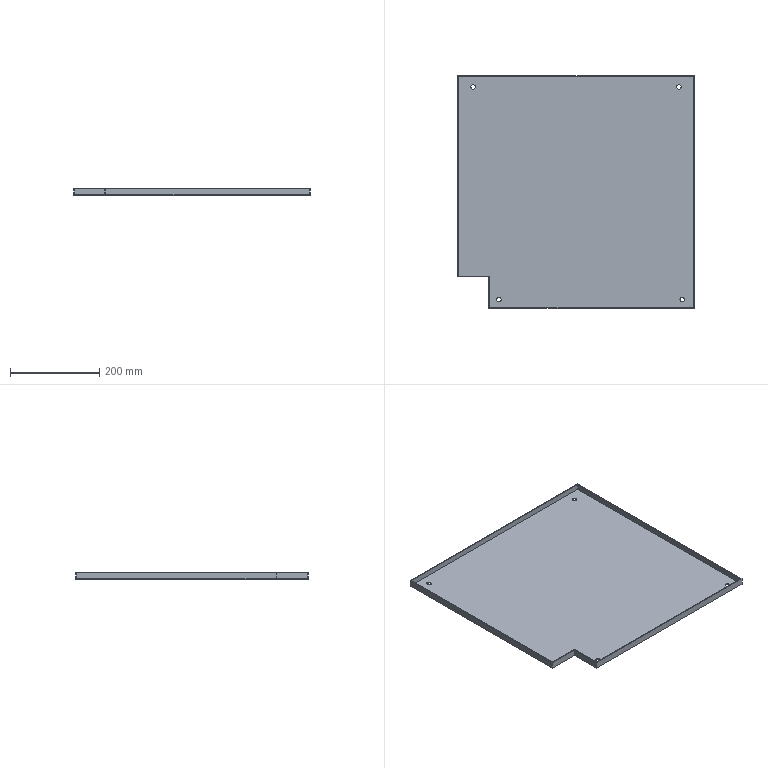Part | STEP file | 11-FGJJ-01411 | 1 solid | 23 faces | box 530 x 520 x 15 mm | volume 595164 mm3 | plane 15 | cylinder 8 | commonest cylinder face diameters 10 x8
STEP:
#1=CARTESIAN_POINT('',(-235.,235.,2.));
#2=VERTEX_POINT('',#1);
#3=CARTESIAN_POINT('',(-225.,235.,2.));
#4=VERTEX_POINT('',#3);
#5=CARTESIAN_POINT('',(-230.,235.,2.));
#6=DIRECTION('',(0.,0.,1.));
#7=DIRECTION('',(1.,0.,0.));
#8=AXIS2_PLACEMENT_3D('',#5,#6,#7);
#9=CIRCLE('',#8,5.);
#10=EDGE_CURVE('',#2,#4,#9,.T.);
#11=ORIENTED_EDGE('',*,*,#10,.T.);
#12=CARTESIAN_POINT('',(-225.,235.,0.));
#13=VERTEX_POINT('',#12);
#14=CARTESIAN_POINT('',(-225.,235.,28.));
#15=DIRECTION('',(0.,0.,-1.));
#16=VECTOR('',#15,1000.);
#17=LINE('',#14,#16);
#18=EDGE_CURVE('',#4,#13,#17,.T.);
#19=ORIENTED_EDGE('',*,*,#18,.T.);
#20=CARTESIAN_POINT('',(-235.,235.,0.));
#21=VERTEX_POINT('',#20);
#22=CARTESIAN_POINT('',(-230.,235.,0.));
#23=DIRECTION('',(0.,0.,-1.));
#24=DIRECTION('',(-1.,0.,0.));
#25=AXIS2_PLACEMENT_3D('',#22,#23,#24);
#26=CIRCLE('',#25,5.);
#27=EDGE_CURVE('',#13,#21,#26,.T.);
#28=ORIENTED_EDGE('',*,*,#27,.T.);
#29=CARTESIAN_POINT('',(-235.,235.,28.));
#30=DIRECTION('',(0.,0.,-1.));
#31=VECTOR('',#30,1000.);
#32=LINE('',#29,#31);
#33=EDGE_CURVE('',#2,#21,#32,.T.);
#34=ORIENTED_EDGE('',*,*,#33,.F.);
#35=EDGE_LOOP('',(#11,#19,#28,#34));
#36=FACE_OUTER_BOUND('',#35,.T.);
#37=CARTESIAN_POINT('',(-230.,235.,28.));
#38=DIRECTION('',(0.,0.,-1.));
#39=DIRECTION('',(-1.,0.,0.));
#40=AXIS2_PLACEMENT_3D('',#37,#38,#39);
#41=CYLINDRICAL_SURFACE('',#40,5.);
#42=ADVANCED_FACE('',(#36),#41,.F.);
#43=CARTESIAN_POINT('',(232.5,-241.,2.));
#44=VERTEX_POINT('',#43);
#45=CARTESIAN_POINT('',(242.5,-241.,2.));
#46=VERTEX_POINT('',#45);
#47=CARTESIAN_POINT('',(237.5,-241.,2.));
#48=DIRECTION('',(0.,0.,1.));
#49=DIRECTION('',(1.,0.,0.));
#50=AXIS2_PLACEMENT_3D('',#47,#48,#49);
#51=CIRCLE('',#50,5.);
#52=EDGE_CURVE('',#44,#46,#51,.T.);
#53=ORIENTED_EDGE('',*,*,#52,.T.);
#54=CARTESIAN_POINT('',(242.5,-241.,0.));
#55=VERTEX_POINT('',#54);
#56=CARTESIAN_POINT('',(242.5,-241.,28.));
#57=DIRECTION('',(0.,0.,-1.));
#58=VECTOR('',#57,1000.);
#59=LINE('',#56,#58);
#60=EDGE_CURVE('',#46,#55,#59,.T.);
#61=ORIENTED_EDGE('',*,*,#60,.T.);
#62=CARTESIAN_POINT('',(232.5,-241.,0.));
#63=VERTEX_POINT('',#62);
#64=CARTESIAN_POINT('',(237.5,-241.,0.));
#65=DIRECTION('',(0.,0.,-1.));
#66=DIRECTION('',(-1.,0.,0.));
#67=AXIS2_PLACEMENT_3D('',#64,#65,#66);
#68=CIRCLE('',#67,5.);
#69=EDGE_CURVE('',#55,#63,#68,.T.);
#70=ORIENTED_EDGE('',*,*,#69,.T.);
#71=CARTESIAN_POINT('',(232.5,-241.,28.));
#72=DIRECTION('',(0.,0.,-1.));
#73=VECTOR('',#72,1000.);
#74=LINE('',#71,#73);
#75=EDGE_CURVE('',#44,#63,#74,.T.);
#76=ORIENTED_EDGE('',*,*,#75,.F.);
#77=EDGE_LOOP('',(#53,#61,#70,#76));
#78=FACE_OUTER_BOUND('',#77,.T.);
#79=CARTESIAN_POINT('',(237.5,-241.,28.));
#80=DIRECTION('',(0.,0.,-1.));
#81=DIRECTION('',(-1.,0.,0.));
#82=AXIS2_PLACEMENT_3D('',#79,#80,#81);
#83=CYLINDRICAL_SURFACE('',#82,5.);
#84=ADVANCED_FACE('',(#78),#83,.F.);
#85=CARTESIAN_POINT('',(-177.5,-241.,2.));
#86=VERTEX_POINT('',#85);
#87=CARTESIAN_POINT('',(-167.5,-241.,2.));
#88=VERTEX_POINT('',#87);
#89=CARTESIAN_POINT('',(-172.5,-241.,2.));
#90=DIRECTION('',(0.,0.,1.));
#91=DIRECTION('',(1.,0.,0.));
#92=AXIS2_PLACEMENT_3D('',#89,#90,#91);
#93=CIRCLE('',#92,5.);
#94=EDGE_CURVE('',#86,#88,#93,.T.);
#95=ORIENTED_EDGE('',*,*,#94,.T.);
#96=CARTESIAN_POINT('',(-167.5,-241.,0.));
#97=VERTEX_POINT('',#96);
#98=CARTESIAN_POINT('',(-167.5,-241.,28.));
#99=DIRECTION('',(0.,0.,-1.));
#100=VECTOR('',#99,1000.);
#101=LINE('',#98,#100);
#102=EDGE_CURVE('',#88,#97,#101,.T.);
#103=ORIENTED_EDGE('',*,*,#102,.T.);
#104=CARTESIAN_POINT('',(-177.5,-241.,0.));
#105=VERTEX_POINT('',#104);
#106=CARTESIAN_POINT('',(-172.5,-241.,0.));
#107=DIRECTION('',(0.,0.,-1.));
#108=DIRECTION('',(-1.,0.,0.));
#109=AXIS2_PLACEMENT_3D('',#106,#107,#108);
#110=CIRCLE('',#109,5.);
#111=EDGE_CURVE('',#97,#105,#110,.T.);
#112=ORIENTED_EDGE('',*,*,#111,.T.);
#113=CARTESIAN_POINT('',(-177.5,-241.,28.));
#114=DIRECTION('',(0.,0.,-1.));
#115=VECTOR('',#114,1000.);
#116=LINE('',#113,#115);
#117=EDGE_CURVE('',#86,#105,#116,.T.);
#118=ORIENTED_EDGE('',*,*,#117,.F.);
#119=EDGE_LOOP('',(#95,#103,#112,#118));
#120=FACE_OUTER_BOUND('',#119,.T.);
#121=CARTESIAN_POINT('',(-172.5,-241.,28.));
#122=DIRECTION('',(0.,0.,-1.));
#123=DIRECTION('',(-1.,0.,0.));
#124=AXIS2_PLACEMENT_3D('',#121,#122,#123);
#125=CYLINDRICAL_SURFACE('',#124,5.);
#126=ADVANCED_FACE('',(#120),#125,.F.);
#127=CARTESIAN_POINT('',(225.,235.,2.));
#128=VERTEX_POINT('',#127);
#129=CARTESIAN_POINT('',(235.,235.,2.));
#130=VERTEX_POINT('',#129);
#131=CARTESIAN_POINT('',(230.,235.,2.));
#132=DIRECTION('',(0.,0.,1.));
#133=DIRECTION('',(1.,0.,0.));
#134=AXIS2_PLACEMENT_3D('',#131,#132,#133);
#135=CIRCLE('',#134,5.);
#136=EDGE_CURVE('',#128,#130,#135,.T.);
#137=ORIENTED_EDGE('',*,*,#136,.T.);
#138=CARTESIAN_POINT('',(235.,235.,0.));
#139=VERTEX_POINT('',#138);
#140=CARTESIAN_POINT('',(235.,235.,28.));
#141=DIRECTION('',(0.,0.,-1.));
#142=VECTOR('',#141,1000.);
#143=LINE('',#140,#142);
#144=EDGE_CURVE('',#130,#139,#143,.T.);
#145=ORIENTED_EDGE('',*,*,#144,.T.);
#146=CARTESIAN_POINT('',(225.,235.,0.));
#147=VERTEX_POINT('',#146);
#148=CARTESIAN_POINT('',(230.,235.,0.));
#149=DIRECTION('',(0.,0.,-1.));
#150=DIRECTION('',(-1.,0.,0.));
#151=AXIS2_PLACEMENT_3D('',#148,#149,#150);
#152=CIRCLE('',#151,5.);
#153=EDGE_CURVE('',#139,#147,#152,.T.);
#154=ORIENTED_EDGE('',*,*,#153,.T.);
#155=CARTESIAN_POINT('',(225.,235.,28.));
#156=DIRECTION('',(0.,0.,-1.));
#157=VECTOR('',#156,1000.);
#158=LINE('',#155,#157);
#159=EDGE_CURVE('',#128,#147,#158,.T.);
#160=ORIENTED_EDGE('',*,*,#159,.F.);
#161=EDGE_LOOP('',(#137,#145,#154,#160));
#162=FACE_OUTER_BOUND('',#161,.T.);
#163=CARTESIAN_POINT('',(230.,235.,28.));
#164=DIRECTION('',(0.,0.,-1.));
#165=DIRECTION('',(-1.,0.,0.));
#166=AXIS2_PLACEMENT_3D('',#163,#164,#165);
#167=CYLINDRICAL_SURFACE('',#166,5.);
#168=ADVANCED_FACE('',(#162),#167,.F.);
#169=CARTESIAN_POINT('',(-263.,258.,15.));
#170=VERTEX_POINT('',#169);
#171=CARTESIAN_POINT('',(-263.,-188.,15.));
#172=VERTEX_POINT('',#171);
#173=CARTESIAN_POINT('',(-263.,260.,15.));
#174=DIRECTION('',(0.,-1.,0.));
#175=VECTOR('',#174,1000.);
#176=LINE('',#173,#175);
#177=EDGE_CURVE('',#170,#172,#176,.T.);
#178=ORIENTED_EDGE('',*,*,#177,.T.);
#179=CARTESIAN_POINT('',(-263.,-188.,2.));
#180=VERTEX_POINT('',#179);
#181=CARTESIAN_POINT('',(-263.,-188.,113.995));
#182=DIRECTION('',(0.,0.,-1.));
#183=VECTOR('',#182,1000.);
#184=LINE('',#181,#183);
#185=EDGE_CURVE('',#172,#180,#184,.T.);
#186=ORIENTED_EDGE('',*,*,#185,.T.);
#187=CARTESIAN_POINT('',(-263.,258.,2.));
#188=VERTEX_POINT('',#187);
#189=CARTESIAN_POINT('',(-263.,260.,2.));
#190=DIRECTION('',(0.,-1.,0.));
#191=VECTOR('',#190,1000.);
#192=LINE('',#189,#191);
#193=EDGE_CURVE('',#188,#180,#192,.T.);
#194=ORIENTED_EDGE('',*,*,#193,.F.);
#195=CARTESIAN_POINT('',(-263.,258.,15.));
#196=DIRECTION('',(0.,0.,-1.));
#197=VECTOR('',#196,1000.);
#198=LINE('',#195,#197);
#199=EDGE_CURVE('',#170,#188,#198,.T.);
#200=ORIENTED_EDGE('',*,*,#199,.F.);
#201=EDGE_LOOP('',(#178,#186,#194,#200));
#202=FACE_OUTER_BOUND('',#201,.T.);
#203=CARTESIAN_POINT('',(-263.,260.,15.));
#204=DIRECTION('',(1.,0.,0.));
#205=DIRECTION('',(0.,1.,0.));
#206=AXIS2_PLACEMENT_3D('',#203,#204,#205);
#207=PLANE('',#206);
#208=ADVANCED_FACE('',(#202),#207,.T.);
#209=CARTESIAN_POINT('',(-193.,-258.,2.));
#210=VERTEX_POINT('',#209);
#211=CARTESIAN_POINT('',(263.,-258.,2.));
#212=VERTEX_POINT('',#211);
#213=CARTESIAN_POINT('',(-265.,-258.,2.));
#214=DIRECTION('',(1.,0.,0.));
#215=VECTOR('',#214,1000.);
#216=LINE('',#213,#215);
#217=EDGE_CURVE('',#210,#212,#216,.T.);
#218=ORIENTED_EDGE('',*,*,#217,.F.);
#219=CARTESIAN_POINT('',(-193.,-258.,15.));
#220=VERTEX_POINT('',#219);
#221=CARTESIAN_POINT('',(-193.,-258.,113.995));
#222=DIRECTION('',(0.,0.,-1.));
#223=VECTOR('',#222,1000.);
#224=LINE('',#221,#223);
#225=EDGE_CURVE('',#220,#210,#224,.T.);
#226=ORIENTED_EDGE('',*,*,#225,.F.);
#227=CARTESIAN_POINT('',(263.,-258.,15.));
#228=VERTEX_POINT('',#227);
#229=CARTESIAN_POINT('',(-265.,-258.,15.));
#230=DIRECTION('',(1.,0.,0.));
#231=VECTOR('',#230,1000.);
#232=LINE('',#229,#231);
#233=EDGE_CURVE('',#220,#228,#232,.T.);
#234=ORIENTED_EDGE('',*,*,#233,.T.);
#235=CARTESIAN_POINT('',(263.,-258.,15.));
#236=DIRECTION('',(0.,0.,-1.));
#237=VECTOR('',#236,1000.);
#238=LINE('',#235,#237);
#239=EDGE_CURVE('',#228,#212,#238,.T.);
#240=ORIENTED_EDGE('',*,*,#239,.T.);
#241=EDGE_LOOP('',(#218,#226,#234,#240));
#242=FACE_OUTER_BOUND('',#241,.T.);
#243=CARTESIAN_POINT('',(-265.,-258.,15.));
#244=DIRECTION('',(0.,1.,0.));
#245=DIRECTION('',(0.,0.,1.));
#246=AXIS2_PLACEMENT_3D('',#243,#244,#245);
#247=PLANE('',#246);
#248=ADVANCED_FACE('',(#242),#247,.T.);
#249=ORIENTED_EDGE('',*,*,#10,.F.);
#250=CARTESIAN_POINT('',(-230.,235.,2.));
#251=DIRECTION('',(0.,0.,1.));
#252=DIRECTION('',(1.,0.,0.));
#253=AXIS2_PLACEMENT_3D('',#250,#251,#252);
#254=CIRCLE('',#253,5.);
#255=EDGE_CURVE('',#4,#2,#254,.T.);
#256=ORIENTED_EDGE('',*,*,#255,.F.);
#257=EDGE_LOOP('',(#249,#256));
#258=FACE_BOUND('',#257,.T.);
#259=ORIENTED_EDGE('',*,*,#52,.F.);
#260=CARTESIAN_POINT('',(237.5,-241.,2.));
#261=DIRECTION('',(0.,0.,1.));
#262=DIRECTION('',(1.,0.,0.));
#263=AXIS2_PLACEMENT_3D('',#260,#261,#262);
#264=CIRCLE('',#263,5.);
#265=EDGE_CURVE('',#46,#44,#264,.T.);
#266=ORIENTED_EDGE('',*,*,#265,.F.);
#267=EDGE_LOOP('',(#259,#266));
#268=FACE_BOUND('',#267,.T.);
#269=ORIENTED_EDGE('',*,*,#94,.F.);
#270=CARTESIAN_POINT('',(-172.5,-241.,2.));
#271=DIRECTION('',(0.,0.,1.));
#272=DIRECTION('',(1.,0.,0.));
#273=AXIS2_PLACEMENT_3D('',#270,#271,#272);
#274=CIRCLE('',#273,5.);
#275=EDGE_CURVE('',#88,#86,#274,.T.);
#276=ORIENTED_EDGE('',*,*,#275,.F.);
#277=EDGE_LOOP('',(#269,#276));
#278=FACE_BOUND('',#277,.T.);
#279=ORIENTED_EDGE('',*,*,#136,.F.);
#280=CARTESIAN_POINT('',(230.,235.,2.));
#281=DIRECTION('',(0.,0.,1.));
#282=DIRECTION('',(1.,0.,0.));
#283=AXIS2_PLACEMENT_3D('',#280,#281,#282);
#284=CIRCLE('',#283,5.);
#285=EDGE_CURVE('',#130,#128,#284,.T.);
#286=ORIENTED_EDGE('',*,*,#285,.F.);
#287=EDGE_LOOP('',(#279,#286));
#288=FACE_BOUND('',#287,.T.);
#289=CARTESIAN_POINT('',(-193.,-188.,2.));
#290=VERTEX_POINT('',#289);
#291=CARTESIAN_POINT('',(-263.,-188.,2.));
#292=DIRECTION('',(-1.,0.,0.));
#293=VECTOR('',#292,1000.);
#294=LINE('',#291,#293);
#295=EDGE_CURVE('',#290,#180,#294,.T.);
#296=ORIENTED_EDGE('',*,*,#295,.F.);
#297=CARTESIAN_POINT('',(-193.,-258.,2.));
#298=DIRECTION('',(0.,1.,0.));
#299=VECTOR('',#298,1000.);
#300=LINE('',#297,#299);
#301=EDGE_CURVE('',#210,#290,#300,.T.);
#302=ORIENTED_EDGE('',*,*,#301,.F.);
#303=ORIENTED_EDGE('',*,*,#217,.T.);
#304=CARTESIAN_POINT('',(263.,258.,2.));
#305=VERTEX_POINT('',#304);
#306=CARTESIAN_POINT('',(263.,260.,2.));
#307=DIRECTION('',(0.,1.,0.));
#308=VECTOR('',#307,1000.);
#309=LINE('',#306,#308);
#310=EDGE_CURVE('',#212,#305,#309,.T.);
#311=ORIENTED_EDGE('',*,*,#310,.T.);
#312=CARTESIAN_POINT('',(-265.,258.,2.));
#313=DIRECTION('',(-1.,0.,0.));
#314=VECTOR('',#313,1000.);
#315=LINE('',#312,#314);
#316=EDGE_CURVE('',#305,#188,#315,.T.);
#317=ORIENTED_EDGE('',*,*,#316,.T.);
#318=ORIENTED_EDGE('',*,*,#193,.T.);
#319=EDGE_LOOP('',(#296,#302,#303,#311,#317,#318));
#320=FACE_OUTER_BOUND('',#319,.T.);
#321=CARTESIAN_POINT('',(0.,0.,2.));
#322=DIRECTION('',(0.,0.,1.));
#323=DIRECTION('',(1.,0.,0.));
#324=AXIS2_PLACEMENT_3D('',#321,#322,#323);
#325=PLANE('',#324);
#326=ADVANCED_FACE('',(#258,#268,#278,#288,#320),#325,.T.);
#327=CARTESIAN_POINT('',(265.,-260.,0.));
#328=VERTEX_POINT('',#327);
#329=CARTESIAN_POINT('',(265.,260.,0.));
#330=VERTEX_POINT('',#329);
#331=CARTESIAN_POINT('',(265.,260.,0.));
#332=DIRECTION('',(0.,1.,0.));
#333=VECTOR('',#332,1000.);
#334=LINE('',#331,#333);
#335=EDGE_CURVE('',#328,#330,#334,.T.);
#336=ORIENTED_EDGE('',*,*,#335,.T.);
#337=CARTESIAN_POINT('',(265.,260.,15.));
#338=VERTEX_POINT('',#337);
#339=CARTESIAN_POINT('',(265.,260.,15.));
#340=DIRECTION('',(0.,0.,-1.));
#341=VECTOR('',#340,1000.);
#342=LINE('',#339,#341);
#343=EDGE_CURVE('',#338,#330,#342,.T.);
#344=ORIENTED_EDGE('',*,*,#343,.F.);
#345=CARTESIAN_POINT('',(265.,-260.,15.));
#346=VERTEX_POINT('',#345);
#347=CARTESIAN_POINT('',(265.,260.,15.));
#348=DIRECTION('',(0.,1.,0.));
#349=VECTOR('',#348,1000.);
#350=LINE('',#347,#349);
#351=EDGE_CURVE('',#346,#338,#350,.T.);
#352=ORIENTED_EDGE('',*,*,#351,.F.);
#353=CARTESIAN_POINT('',(265.,-260.,15.));
#354=DIRECTION('',(0.,0.,-1.));
#355=VECTOR('',#354,1000.);
#356=LINE('',#353,#355);
#357=EDGE_CURVE('',#346,#328,#356,.T.);
#358=ORIENTED_EDGE('',*,*,#357,.T.);
#359=EDGE_LOOP('',(#336,#344,#352,#358));
#360=FACE_OUTER_BOUND('',#359,.T.);
#361=CARTESIAN_POINT('',(265.,260.,15.));
#362=DIRECTION('',(-1.,0.,0.));
#363=DIRECTION('',(0.,-1.,0.));
#364=AXIS2_PLACEMENT_3D('',#361,#362,#363);
#365=PLANE('',#364);
#366=ADVANCED_FACE('',(#360),#365,.F.);
#367=CARTESIAN_POINT('',(-265.,260.,0.));
#368=VERTEX_POINT('',#367);
#369=CARTESIAN_POINT('',(-265.,260.,0.));
#370=DIRECTION('',(-1.,0.,0.));
#371=VECTOR('',#370,1000.);
#372=LINE('',#369,#371);
#373=EDGE_CURVE('',#330,#368,#372,.T.);
#374=ORIENTED_EDGE('',*,*,#373,.T.);
#375=CARTESIAN_POINT('',(-265.,260.,15.));
#376=VERTEX_POINT('',#375);
#377=CARTESIAN_POINT('',(-265.,260.,15.));
#378=DIRECTION('',(0.,0.,-1.));
#379=VECTOR('',#378,1000.);
#380=LINE('',#377,#379);
#381=EDGE_CURVE('',#376,#368,#380,.T.);
#382=ORIENTED_EDGE('',*,*,#381,.F.);
#383=CARTESIAN_POINT('',(-265.,260.,15.));
#384=DIRECTION('',(-1.,0.,0.));
#385=VECTOR('',#384,1000.);
#386=LINE('',#383,#385);
#387=EDGE_CURVE('',#338,#376,#386,.T.);
#388=ORIENTED_EDGE('',*,*,#387,.F.);
#389=ORIENTED_EDGE('',*,*,#343,.T.);
#390=EDGE_LOOP('',(#374,#382,#388,#389));
#391=FACE_OUTER_BOUND('',#390,.T.);
#392=CARTESIAN_POINT('',(-265.,260.,15.));
#393=DIRECTION('',(0.,-1.,0.));
#394=DIRECTION('',(0.,0.,-1.));
#395=AXIS2_PLACEMENT_3D('',#392,#393,#394);
#396=PLANE('',#395);
#397=ADVANCED_FACE('',(#391),#396,.F.);
#398=CARTESIAN_POINT('',(-265.,-190.,0.));
#399=VERTEX_POINT('',#398);
#400=CARTESIAN_POINT('',(-265.,260.,0.));
#401=DIRECTION('',(0.,-1.,0.));
#402=VECTOR('',#401,1000.);
#403=LINE('',#400,#402);
#404=EDGE_CURVE('',#368,#399,#403,.T.);
#405=ORIENTED_EDGE('',*,*,#404,.T.);
#406=CARTESIAN_POINT('',(-265.,-190.,15.));
#407=VERTEX_POINT('',#406);
#408=CARTESIAN_POINT('',(-265.,-190.,28.));
#409=DIRECTION('',(0.,0.,-1.));
#410=VECTOR('',#409,1000.);
#411=LINE('',#408,#410);
#412=EDGE_CURVE('',#407,#399,#411,.T.);
#413=ORIENTED_EDGE('',*,*,#412,.F.);
#414=CARTESIAN_POINT('',(-265.,260.,15.));
#415=DIRECTION('',(0.,-1.,0.));
#416=VECTOR('',#415,1000.);
#417=LINE('',#414,#416);
#418=EDGE_CURVE('',#376,#407,#417,.T.);
#419=ORIENTED_EDGE('',*,*,#418,.F.);
#420=ORIENTED_EDGE('',*,*,#381,.T.);
#421=EDGE_LOOP('',(#405,#413,#419,#420));
#422=FACE_OUTER_BOUND('',#421,.T.);
#423=CARTESIAN_POINT('',(-265.,260.,15.));
#424=DIRECTION('',(1.,0.,0.));
#425=DIRECTION('',(0.,1.,0.));
#426=AXIS2_PLACEMENT_3D('',#423,#424,#425);
#427=PLANE('',#426);
#428=ADVANCED_FACE('',(#422),#427,.F.);
#429=CARTESIAN_POINT('',(-195.,-260.,15.));
#430=VERTEX_POINT('',#429);
#431=CARTESIAN_POINT('',(-265.,-260.,15.));
#432=DIRECTION('',(1.,0.,0.));
#433=VECTOR('',#432,1000.);
#434=LINE('',#431,#433);
#435=EDGE_CURVE('',#430,#346,#434,.T.);
#436=ORIENTED_EDGE('',*,*,#435,.F.);
#437=CARTESIAN_POINT('',(-195.,-260.,0.));
#438=VERTEX_POINT('',#437);
#439=CARTESIAN_POINT('',(-195.,-260.,28.));
#440=DIRECTION('',(0.,0.,-1.));
#441=VECTOR('',#440,1000.);
#442=LINE('',#439,#441);
#443=EDGE_CURVE('',#430,#438,#442,.T.);
#444=ORIENTED_EDGE('',*,*,#443,.T.);
#445=CARTESIAN_POINT('',(-265.,-260.,0.));
#446=DIRECTION('',(1.,0.,0.));
#447=VECTOR('',#446,1000.);
#448=LINE('',#445,#447);
#449=EDGE_CURVE('',#438,#328,#448,.T.);
#450=ORIENTED_EDGE('',*,*,#449,.T.);
#451=ORIENTED_EDGE('',*,*,#357,.F.);
#452=EDGE_LOOP('',(#436,#444,#450,#451));
#453=FACE_OUTER_BOUND('',#452,.T.);
#454=CARTESIAN_POINT('',(-265.,-260.,15.));
#455=DIRECTION('',(0.,1.,0.));
#456=DIRECTION('',(0.,0.,1.));
#457=AXIS2_PLACEMENT_3D('',#454,#455,#456);
#458=PLANE('',#457);
#459=ADVANCED_FACE('',(#453),#458,.F.);
#460=CARTESIAN_POINT('',(-195.,-190.,15.));
#461=VERTEX_POINT('',#460);
#462=CARTESIAN_POINT('',(0.,-190.,15.));
#463=DIRECTION('',(-1.,0.,0.));
#464=VECTOR('',#463,1000.);
#465=LINE('',#462,#464);
#466=EDGE_CURVE('',#461,#407,#465,.T.);
#467=ORIENTED_EDGE('',*,*,#466,.F.);
#468=CARTESIAN_POINT('',(-195.,0.,15.));
#469=DIRECTION('',(0.,1.,0.));
#470=VECTOR('',#469,1000.);
#471=LINE('',#468,#470);
#472=EDGE_CURVE('',#430,#461,#471,.T.);
#473=ORIENTED_EDGE('',*,*,#472,.F.);
#474=ORIENTED_EDGE('',*,*,#435,.T.);
#475=ORIENTED_EDGE('',*,*,#351,.T.);
#476=ORIENTED_EDGE('',*,*,#387,.T.);
#477=ORIENTED_EDGE('',*,*,#418,.T.);
#478=EDGE_LOOP('',(#467,#473,#474,#475,#476,#477));
#479=FACE_OUTER_BOUND('',#478,.T.);
#480=CARTESIAN_POINT('',(-193.,-188.,15.));
#481=VERTEX_POINT('',#480);
#482=CARTESIAN_POINT('',(-263.,-188.,15.));
#483=DIRECTION('',(-1.,0.,0.));
#484=VECTOR('',#483,1000.);
#485=LINE('',#482,#484);
#486=EDGE_CURVE('',#481,#172,#485,.T.);
#487=ORIENTED_EDGE('',*,*,#486,.T.);
#488=ORIENTED_EDGE('',*,*,#177,.F.);
#489=CARTESIAN_POINT('',(263.,258.,15.));
#490=VERTEX_POINT('',#489);
#491=CARTESIAN_POINT('',(-265.,258.,15.));
#492=DIRECTION('',(-1.,0.,0.));
#493=VECTOR('',#492,1000.);
#494=LINE('',#491,#493);
#495=EDGE_CURVE('',#490,#170,#494,.T.);
#496=ORIENTED_EDGE('',*,*,#495,.F.);
#497=CARTESIAN_POINT('',(263.,260.,15.));
#498=DIRECTION('',(0.,1.,0.));
#499=VECTOR('',#498,1000.);
#500=LINE('',#497,#499);
#501=EDGE_CURVE('',#228,#490,#500,.T.);
#502=ORIENTED_EDGE('',*,*,#501,.F.);
#503=ORIENTED_EDGE('',*,*,#233,.F.);
#504=CARTESIAN_POINT('',(-193.,-258.,15.));
#505=DIRECTION('',(0.,1.,0.));
#506=VECTOR('',#505,1000.);
#507=LINE('',#504,#506);
#508=EDGE_CURVE('',#220,#481,#507,.T.);
#509=ORIENTED_EDGE('',*,*,#508,.T.);
#510=EDGE_LOOP('',(#487,#488,#496,#502,#503,#509));
#511=FACE_BOUND('',#510,.T.);
#512=CARTESIAN_POINT('',(0.,0.,15.));
#513=DIRECTION('',(0.,0.,1.));
#514=DIRECTION('',(1.,0.,0.));
#515=AXIS2_PLACEMENT_3D('',#512,#513,#514);
#516=PLANE('',#515);
#517=ADVANCED_FACE('',(#479,#511),#516,.T.);
#518=CARTESIAN_POINT('',(-230.,235.,0.));
#519=DIRECTION('',(0.,0.,-1.));
#520=DIRECTION('',(-1.,0.,0.));
#521=AXIS2_PLACEMENT_3D('',#518,#519,#520);
#522=CIRCLE('',#521,5.);
#523=EDGE_CURVE('',#21,#13,#522,.T.);
#524=ORIENTED_EDGE('',*,*,#523,.F.);
#525=ORIENTED_EDGE('',*,*,#27,.F.);
#526=EDGE_LOOP('',(#524,#525));
#527=FACE_BOUND('',#526,.T.);
#528=CARTESIAN_POINT('',(237.5,-241.,0.));
#529=DIRECTION('',(0.,0.,-1.));
#530=DIRECTION('',(-1.,0.,0.));
#531=AXIS2_PLACEMENT_3D('',#528,#529,#530);
#532=CIRCLE('',#531,5.);
#533=EDGE_CURVE('',#63,#55,#532,.T.);
#534=ORIENTED_EDGE('',*,*,#533,.F.);
#535=ORIENTED_EDGE('',*,*,#69,.F.);
#536=EDGE_LOOP('',(#534,#535));
#537=FACE_BOUND('',#536,.T.);
#538=CARTESIAN_POINT('',(-172.5,-241.,0.));
#539=DIRECTION('',(0.,0.,-1.));
#540=DIRECTION('',(-1.,0.,0.));
#541=AXIS2_PLACEMENT_3D('',#538,#539,#540);
#542=CIRCLE('',#541,5.);
#543=EDGE_CURVE('',#105,#97,#542,.T.);
#544=ORIENTED_EDGE('',*,*,#543,.F.);
#545=ORIENTED_EDGE('',*,*,#111,.F.);
#546=EDGE_LOOP('',(#544,#545));
#547=FACE_BOUND('',#546,.T.);
#548=CARTESIAN_POINT('',(230.,235.,0.));
#549=DIRECTION('',(0.,0.,-1.));
#550=DIRECTION('',(-1.,0.,0.));
#551=AXIS2_PLACEMENT_3D('',#548,#549,#550);
#552=CIRCLE('',#551,5.);
#553=EDGE_CURVE('',#147,#139,#552,.T.);
#554=ORIENTED_EDGE('',*,*,#553,.F.);
#555=ORIENTED_EDGE('',*,*,#153,.F.);
#556=EDGE_LOOP('',(#554,#555));
#557=FACE_BOUND('',#556,.T.);
#558=ORIENTED_EDGE('',*,*,#449,.F.);
#559=CARTESIAN_POINT('',(-195.,-190.,0.));
#560=VERTEX_POINT('',#559);
#561=CARTESIAN_POINT('',(-195.,-260.,0.));
#562=DIRECTION('',(0.,-1.,0.));
#563=VECTOR('',#562,1000.);
#564=LINE('',#561,#563);
#565=EDGE_CURVE('',#560,#438,#564,.T.);
#566=ORIENTED_EDGE('',*,*,#565,.F.);
#567=CARTESIAN_POINT('',(-265.,-190.,0.));
#568=DIRECTION('',(1.,0.,0.));
#569=VECTOR('',#568,1000.);
#570=LINE('',#567,#569);
#571=EDGE_CURVE('',#399,#560,#570,.T.);
#572=ORIENTED_EDGE('',*,*,#571,.F.);
#573=ORIENTED_EDGE('',*,*,#404,.F.);
#574=ORIENTED_EDGE('',*,*,#373,.F.);
#575=ORIENTED_EDGE('',*,*,#335,.F.);
#576=EDGE_LOOP('',(#558,#566,#572,#573,#574,#575));
#577=FACE_OUTER_BOUND('',#576,.T.);
#578=CARTESIAN_POINT('',(0.,0.,0.));
#579=DIRECTION('',(0.,0.,1.));
#580=DIRECTION('',(1.,0.,0.));
#581=AXIS2_PLACEMENT_3D('',#578,#579,#580);
#582=PLANE('',#581);
#583=ADVANCED_FACE('',(#527,#537,#547,#557,#577),#582,.F.);
#584=ORIENTED_EDGE('',*,*,#310,.F.);
#585=ORIENTED_EDGE('',*,*,#239,.F.);
#586=ORIENTED_EDGE('',*,*,#501,.T.);
#587=CARTESIAN_POINT('',(263.,258.,15.));
#588=DIRECTION('',(0.,0.,-1.));
#589=VECTOR('',#588,1000.);
#590=LINE('',#587,#589);
#591=EDGE_CURVE('',#490,#305,#590,.T.);
#592=ORIENTED_EDGE('',*,*,#591,.T.);
#593=EDGE_LOOP('',(#584,#585,#586,#592));
#594=FACE_OUTER_BOUND('',#593,.T.);
#595=CARTESIAN_POINT('',(263.,260.,15.));
#596=DIRECTION('',(-1.,0.,0.));
#597=DIRECTION('',(0.,-1.,0.));
#598=AXIS2_PLACEMENT_3D('',#595,#596,#597);
#599=PLANE('',#598);
#600=ADVANCED_FACE('',(#594),#599,.T.);
#601=ORIENTED_EDGE('',*,*,#316,.F.);
#602=ORIENTED_EDGE('',*,*,#591,.F.);
#603=ORIENTED_EDGE('',*,*,#495,.T.);
#604=ORIENTED_EDGE('',*,*,#199,.T.);
#605=EDGE_LOOP('',(#601,#602,#603,#604));
#606=FACE_OUTER_BOUND('',#605,.T.);
#607=CARTESIAN_POINT('',(-265.,258.,15.));
#608=DIRECTION('',(0.,-1.,0.));
#609=DIRECTION('',(0.,0.,-1.));
#610=AXIS2_PLACEMENT_3D('',#607,#608,#609);
#611=PLANE('',#610);
#612=ADVANCED_FACE('',(#606),#611,.T.);
#613=ORIENTED_EDGE('',*,*,#144,.F.);
#614=ORIENTED_EDGE('',*,*,#285,.T.);
#615=ORIENTED_EDGE('',*,*,#159,.T.);
#616=ORIENTED_EDGE('',*,*,#553,.T.);
#617=EDGE_LOOP('',(#613,#614,#615,#616));
#618=FACE_OUTER_BOUND('',#617,.T.);
#619=CARTESIAN_POINT('',(230.,235.,28.));
#620=DIRECTION('',(0.,0.,-1.));
#621=DIRECTION('',(-1.,0.,0.));
#622=AXIS2_PLACEMENT_3D('',#619,#620,#621);
#623=CYLINDRICAL_SURFACE('',#622,5.);
#624=ADVANCED_FACE('',(#618),#623,.F.);
#625=ORIENTED_EDGE('',*,*,#102,.F.);
#626=ORIENTED_EDGE('',*,*,#275,.T.);
#627=ORIENTED_EDGE('',*,*,#117,.T.);
#628=ORIENTED_EDGE('',*,*,#543,.T.);
#629=EDGE_LOOP('',(#625,#626,#627,#628));
#630=FACE_OUTER_BOUND('',#629,.T.);
#631=CARTESIAN_POINT('',(-172.5,-241.,28.));
#632=DIRECTION('',(0.,0.,-1.));
#633=DIRECTION('',(-1.,0.,0.));
#634=AXIS2_PLACEMENT_3D('',#631,#632,#633);
#635=CYLINDRICAL_SURFACE('',#634,5.);
#636=ADVANCED_FACE('',(#630),#635,.F.);
#637=ORIENTED_EDGE('',*,*,#60,.F.);
#638=ORIENTED_EDGE('',*,*,#265,.T.);
#639=ORIENTED_EDGE('',*,*,#75,.T.);
#640=ORIENTED_EDGE('',*,*,#533,.T.);
#641=EDGE_LOOP('',(#637,#638,#639,#640));
#642=FACE_OUTER_BOUND('',#641,.T.);
#643=CARTESIAN_POINT('',(237.5,-241.,28.));
#644=DIRECTION('',(0.,0.,-1.));
#645=DIRECTION('',(-1.,0.,0.));
#646=AXIS2_PLACEMENT_3D('',#643,#644,#645);
#647=CYLINDRICAL_SURFACE('',#646,5.);
#648=ADVANCED_FACE('',(#642),#647,.F.);
#649=ORIENTED_EDGE('',*,*,#18,.F.);
#650=ORIENTED_EDGE('',*,*,#255,.T.);
#651=ORIENTED_EDGE('',*,*,#33,.T.);
#652=ORIENTED_EDGE('',*,*,#523,.T.);
#653=EDGE_LOOP('',(#649,#650,#651,#652));
#654=FACE_OUTER_BOUND('',#653,.T.);
#655=CARTESIAN_POINT('',(-230.,235.,28.));
#656=DIRECTION('',(0.,0.,-1.));
#657=DIRECTION('',(-1.,0.,0.));
#658=AXIS2_PLACEMENT_3D('',#655,#656,#657);
#659=CYLINDRICAL_SURFACE('',#658,5.);
#660=ADVANCED_FACE('',(#654),#659,.F.);
#661=ORIENTED_EDGE('',*,*,#472,.T.);
#662=CARTESIAN_POINT('',(-195.,-190.,28.));
#663=DIRECTION('',(0.,0.,-1.));
#664=VECTOR('',#663,1000.);
#665=LINE('',#662,#664);
#666=EDGE_CURVE('',#461,#560,#665,.T.);
#667=ORIENTED_EDGE('',*,*,#666,.T.);
#668=ORIENTED_EDGE('',*,*,#565,.T.);
#669=ORIENTED_EDGE('',*,*,#443,.F.);
#670=EDGE_LOOP('',(#661,#667,#668,#669));
#671=FACE_OUTER_BOUND('',#670,.T.);
#672=CARTESIAN_POINT('',(-195.,-260.,28.));
#673=DIRECTION('',(1.,0.,0.));
#674=DIRECTION('',(0.,0.,-1.));
#675=AXIS2_PLACEMENT_3D('',#672,#673,#674);
#676=PLANE('',#675);
#677=ADVANCED_FACE('',(#671),#676,.F.);
#678=ORIENTED_EDGE('',*,*,#666,.F.);
#679=ORIENTED_EDGE('',*,*,#466,.T.);
#680=ORIENTED_EDGE('',*,*,#412,.T.);
#681=ORIENTED_EDGE('',*,*,#571,.T.);
#682=EDGE_LOOP('',(#678,#679,#680,#681));
#683=FACE_OUTER_BOUND('',#682,.T.);
#684=CARTESIAN_POINT('',(-265.,-190.,28.));
#685=DIRECTION('',(0.,1.,0.));
#686=DIRECTION('',(0.,0.,1.));
#687=AXIS2_PLACEMENT_3D('',#684,#685,#686);
#688=PLANE('',#687);
#689=ADVANCED_FACE('',(#683),#688,.F.);
#690=ORIENTED_EDGE('',*,*,#508,.F.);
#691=ORIENTED_EDGE('',*,*,#225,.T.);
#692=ORIENTED_EDGE('',*,*,#301,.T.);
#693=CARTESIAN_POINT('',(-193.,-188.,113.995));
#694=DIRECTION('',(0.,0.,-1.));
#695=VECTOR('',#694,1000.);
#696=LINE('',#693,#695);
#697=EDGE_CURVE('',#481,#290,#696,.T.);
#698=ORIENTED_EDGE('',*,*,#697,.F.);
#699=EDGE_LOOP('',(#690,#691,#692,#698));
#700=FACE_OUTER_BOUND('',#699,.T.);
#701=CARTESIAN_POINT('',(-193.,-258.,113.995));
#702=DIRECTION('',(-1.,0.,0.));
#703=DIRECTION('',(0.,0.,1.));
#704=AXIS2_PLACEMENT_3D('',#701,#702,#703);
#705=PLANE('',#704);
#706=ADVANCED_FACE('',(#700),#705,.F.);
#707=ORIENTED_EDGE('',*,*,#486,.F.);
#708=ORIENTED_EDGE('',*,*,#697,.T.);
#709=ORIENTED_EDGE('',*,*,#295,.T.);
#710=ORIENTED_EDGE('',*,*,#185,.F.);
#711=EDGE_LOOP('',(#707,#708,#709,#710));
#712=FACE_OUTER_BOUND('',#711,.T.);
#713=CARTESIAN_POINT('',(-263.,-188.,113.995));
#714=DIRECTION('',(0.,-1.,0.));
#715=DIRECTION('',(0.,0.,-1.));
#716=AXIS2_PLACEMENT_3D('',#713,#714,#715);
#717=PLANE('',#716);
#718=ADVANCED_FACE('',(#712),#717,.F.);
#719=CLOSED_SHELL('',(#42,#84,#126,#168,#208,#248,#326,#366,#397,#428,#459,#517,#583,#600,#612,#624,#636,#648,#660,#677,#689,#706,#718));
#720=MANIFOLD_SOLID_BREP('',#719);
#721=CARTESIAN_POINT('',(0.,0.,0.));
#722=DIRECTION('',(0.,0.,1.));
#723=DIRECTION('',(1.,0.,0.));
#724=AXIS2_PLACEMENT_3D('',#721,#722,#723);
#725=(LENGTH_UNIT()NAMED_UNIT(*)SI_UNIT(.MILLI.,.METRE.));
#726=UNCERTAINTY_MEASURE_WITH_UNIT(LENGTH_MEASURE(0.00001),#725,'','');
#727=(NAMED_UNIT(*)PLANE_ANGLE_UNIT()SI_UNIT($,.RADIAN.));
#728=(NAMED_UNIT(*)SI_UNIT($,.STERADIAN.)SOLID_ANGLE_UNIT());
#729=(GEOMETRIC_REPRESENTATION_CONTEXT(3)GLOBAL_UNCERTAINTY_ASSIGNED_CONTEXT((#726))GLOBAL_UNIT_ASSIGNED_CONTEXT((#725,#727,#728))REPRESENTATION_CONTEXT('',''));
#730=ADVANCED_BREP_SHAPE_REPRESENTATION('',(#720,#724),#729);